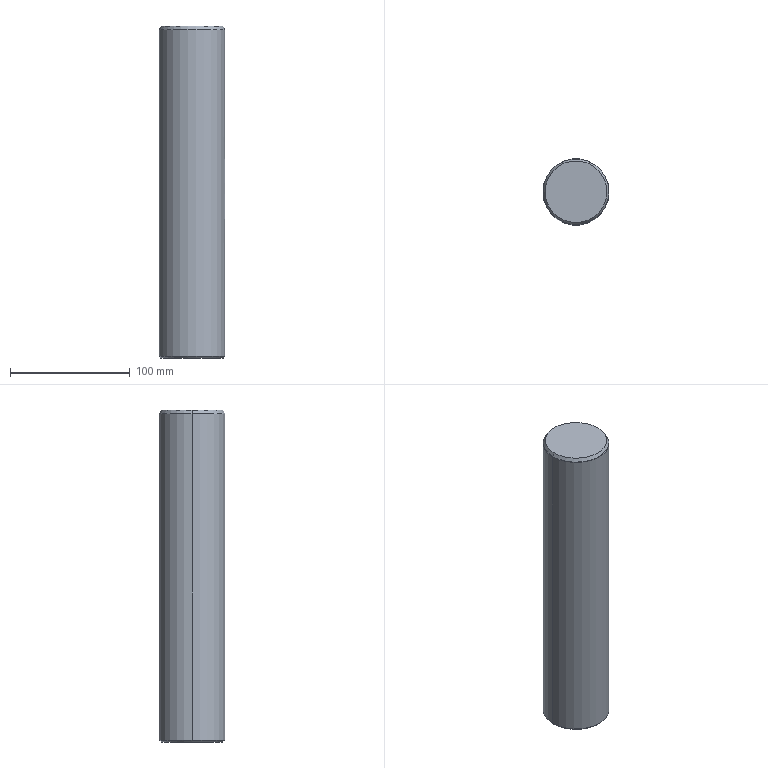Part | SolidWorks | features Chamfer 2, HoleWzd 2, Extrusion 1, Fillet 1 | 1 solid | 22 faces | box 55 x 55 x 277 mm | volume 656436 mm3 | cone 10 | cylinder 8 | torus 2 | plane 2 | commonest cylinder face diameters 6 x4 8 x2 55 x2
STEP:
#1=CARTESIAN_POINT('',(-27.5,0.,273.866));
#2=VERTEX_POINT('',#1);
#3=CARTESIAN_POINT('',(27.5,0.,273.866));
#4=VERTEX_POINT('',#3);
#5=CARTESIAN_POINT('',(0.,0.,273.866));
#6=DIRECTION('',(0.,0.,-1.));
#7=DIRECTION('',(1.,0.,0.));
#8=AXIS2_PLACEMENT_3D('',#5,#6,#7);
#9=CIRCLE('',#8,27.5);
#10=EDGE_CURVE('',#2,#4,#9,.T.);
#11=ORIENTED_EDGE('',*,*,#10,.F.);
#12=CARTESIAN_POINT('',(-27.433,0.,274.116));
#13=VERTEX_POINT('',#12);
#14=CARTESIAN_POINT('',(-27.,0.,273.866));
#15=DIRECTION('',(0.,1.,0.));
#16=DIRECTION('',(-1.,0.,0.));
#17=AXIS2_PLACEMENT_3D('',#14,#15,#16);
#18=CIRCLE('',#17,0.5);
#19=EDGE_CURVE('',#2,#13,#18,.T.);
#20=ORIENTED_EDGE('',*,*,#19,.T.);
#21=CARTESIAN_POINT('',(27.433,0.,274.116));
#22=VERTEX_POINT('',#21);
#23=CARTESIAN_POINT('',(0.,0.,274.116));
#24=DIRECTION('',(0.,0.,1.));
#25=DIRECTION('',(-1.,0.,0.));
#26=AXIS2_PLACEMENT_3D('',#23,#24,#25);
#27=CIRCLE('',#26,27.433);
#28=EDGE_CURVE('',#22,#13,#27,.T.);
#29=ORIENTED_EDGE('',*,*,#28,.F.);
#30=CARTESIAN_POINT('',(27.,0.,273.866));
#31=DIRECTION('',(0.,-1.,0.));
#32=DIRECTION('',(0.,0.,-1.));
#33=AXIS2_PLACEMENT_3D('',#30,#31,#32);
#34=CIRCLE('',#33,0.5);
#35=EDGE_CURVE('',#4,#22,#34,.T.);
#36=ORIENTED_EDGE('',*,*,#35,.F.);
#37=EDGE_LOOP('',(#11,#20,#29,#36));
#38=FACE_OUTER_BOUND('',#37,.T.);
#39=CARTESIAN_POINT('',(0.,0.,273.866));
#40=DIRECTION('',(0.,0.,1.));
#41=DIRECTION('',(1.,0.,0.));
#42=AXIS2_PLACEMENT_3D('',#39,#40,#41);
#43=TOROIDAL_SURFACE('',#42,27.,0.5);
#44=ADVANCED_FACE('',(#38),#43,.T.);
#45=CARTESIAN_POINT('',(25.768,0.,277.));
#46=VERTEX_POINT('',#45);
#47=CARTESIAN_POINT('',(-25.768,0.,277.));
#48=VERTEX_POINT('',#47);
#49=CARTESIAN_POINT('',(0.,0.,277.));
#50=DIRECTION('',(0.,0.,1.));
#51=DIRECTION('',(1.,0.,0.));
#52=AXIS2_PLACEMENT_3D('',#49,#50,#51);
#53=CIRCLE('',#52,25.768);
#54=EDGE_CURVE('',#46,#48,#53,.T.);
#55=ORIENTED_EDGE('',*,*,#54,.F.);
#56=CARTESIAN_POINT('',(25.768,0.,277.));
#57=DIRECTION('',(0.5,0.,-0.866));
#58=VECTOR('',#57,1000.);
#59=LINE('',#56,#58);
#60=EDGE_CURVE('',#46,#22,#59,.T.);
#61=ORIENTED_EDGE('',*,*,#60,.T.);
#62=ORIENTED_EDGE('',*,*,#28,.T.);
#63=CARTESIAN_POINT('',(-25.768,0.,277.));
#64=DIRECTION('',(-0.5,0.,-0.866));
#65=VECTOR('',#64,1000.);
#66=LINE('',#63,#65);
#67=EDGE_CURVE('',#48,#13,#66,.T.);
#68=ORIENTED_EDGE('',*,*,#67,.F.);
#69=EDGE_LOOP('',(#55,#61,#62,#68));
#70=FACE_OUTER_BOUND('',#69,.T.);
#71=CARTESIAN_POINT('',(0.,0.,277.));
#72=DIRECTION('',(0.,0.,-1.));
#73=DIRECTION('',(-1.,0.,0.));
#74=AXIS2_PLACEMENT_3D('',#71,#72,#73);
#75=CONICAL_SURFACE('',#74,25.768,0.5236);
#76=ADVANCED_FACE('',(#70),#75,.T.);
#77=CARTESIAN_POINT('',(-26.,0.,0.));
#78=VERTEX_POINT('',#77);
#79=CARTESIAN_POINT('',(26.,0.,0.));
#80=VERTEX_POINT('',#79);
#81=CARTESIAN_POINT('',(0.,0.,0.));
#82=DIRECTION('',(0.,0.,-1.));
#83=DIRECTION('',(1.,0.,0.));
#84=AXIS2_PLACEMENT_3D('',#81,#82,#83);
#85=CIRCLE('',#84,26.);
#86=EDGE_CURVE('',#78,#80,#85,.T.);
#87=ORIENTED_EDGE('',*,*,#86,.F.);
#88=CARTESIAN_POINT('',(-27.5,0.,1.5));
#89=VERTEX_POINT('',#88);
#90=CARTESIAN_POINT('',(-27.5,0.,1.5));
#91=DIRECTION('',(-0.7071,0.,0.7071));
#92=VECTOR('',#91,1000.);
#93=LINE('',#90,#92);
#94=EDGE_CURVE('',#78,#89,#93,.T.);
#95=ORIENTED_EDGE('',*,*,#94,.T.);
#96=CARTESIAN_POINT('',(27.5,0.,1.5));
#97=VERTEX_POINT('',#96);
#98=CARTESIAN_POINT('',(0.,0.,1.5));
#99=DIRECTION('',(0.,0.,1.));
#100=DIRECTION('',(1.,0.,0.));
#101=AXIS2_PLACEMENT_3D('',#98,#99,#100);
#102=CIRCLE('',#101,27.5);
#103=EDGE_CURVE('',#97,#89,#102,.T.);
#104=ORIENTED_EDGE('',*,*,#103,.F.);
#105=CARTESIAN_POINT('',(27.5,0.,1.5));
#106=DIRECTION('',(0.7071,0.,0.7071));
#107=VECTOR('',#106,1000.);
#108=LINE('',#105,#107);
#109=EDGE_CURVE('',#80,#97,#108,.T.);
#110=ORIENTED_EDGE('',*,*,#109,.F.);
#111=EDGE_LOOP('',(#87,#95,#104,#110));
#112=FACE_OUTER_BOUND('',#111,.T.);
#113=CARTESIAN_POINT('',(0.,0.,1.5));
#114=DIRECTION('',(0.,0.,1.));
#115=DIRECTION('',(1.,0.,0.));
#116=AXIS2_PLACEMENT_3D('',#113,#114,#115);
#117=CONICAL_SURFACE('',#116,27.5,0.7854);
#118=ADVANCED_FACE('',(#112),#117,.T.);
#119=CARTESIAN_POINT('',(17.097,0.,142.));
#120=VERTEX_POINT('',#119);
#121=CARTESIAN_POINT('',(19.5,0.,138.));
#122=VERTEX_POINT('',#121);
#123=CARTESIAN_POINT('',(19.5,0.,138.));
#124=DIRECTION('',(0.515,0.,-0.8572));
#125=VECTOR('',#124,1000.);
#126=LINE('',#123,#125);
#127=EDGE_CURVE('',#120,#122,#126,.T.);
#128=ORIENTED_EDGE('',*,*,#127,.F.);
#129=CARTESIAN_POINT('',(19.5,0.,146.));
#130=VERTEX_POINT('',#129);
#131=CARTESIAN_POINT('',(19.5,0.,146.));
#132=DIRECTION('',(0.515,0.,0.8572));
#133=VECTOR('',#132,1000.);
#134=LINE('',#131,#133);
#135=EDGE_CURVE('',#120,#130,#134,.T.);
#136=ORIENTED_EDGE('',*,*,#135,.T.);
#137=CARTESIAN_POINT('',(19.5,0.,142.));
#138=DIRECTION('',(1.,0.,0.));
#139=DIRECTION('',(0.,0.,-1.));
#140=AXIS2_PLACEMENT_3D('',#137,#138,#139);
#141=CIRCLE('',#140,4.);
#142=EDGE_CURVE('',#130,#122,#141,.T.);
#143=ORIENTED_EDGE('',*,*,#142,.T.);
#144=EDGE_LOOP('',(#128,#136,#143));
#145=FACE_OUTER_BOUND('',#144,.T.);
#146=CARTESIAN_POINT('',(19.5,0.,142.));
#147=DIRECTION('',(1.,0.,0.));
#148=DIRECTION('',(0.,0.,-1.));
#149=AXIS2_PLACEMENT_3D('',#146,#147,#148);
#150=CONICAL_SURFACE('',#149,4.,1.03);
#151=ADVANCED_FACE('',(#145),#150,.F.);
#152=ORIENTED_EDGE('',*,*,#142,.F.);
#153=CARTESIAN_POINT('',(27.5,0.,146.));
#154=VERTEX_POINT('',#153);
#155=CARTESIAN_POINT('',(27.5,0.,146.));
#156=DIRECTION('',(1.,0.,0.));
#157=VECTOR('',#156,1000.);
#158=LINE('',#155,#157);
#159=EDGE_CURVE('',#130,#154,#158,.T.);
#160=ORIENTED_EDGE('',*,*,#159,.T.);
#161=CARTESIAN_POINT('',(27.5,0.,138.));
#162=VERTEX_POINT('',#161);
#163=CARTESIAN_POINT('',(27.5,0.,138.));
#164=CARTESIAN_POINT('',(27.5,-0.2647,138.));
#165=CARTESIAN_POINT('',(27.496,-0.5248,138.026));
#166=CARTESIAN_POINT('',(27.482,-1.037,138.128));
#167=CARTESIAN_POINT('',(27.471,-1.291,138.205));
#168=CARTESIAN_POINT('',(27.444,-1.775,138.406));
#169=CARTESIAN_POINT('',(27.428,-2.005,138.529));
#170=CARTESIAN_POINT('',(27.392,-2.439,138.819));
#171=CARTESIAN_POINT('',(27.373,-2.645,138.988));
#172=CARTESIAN_POINT('',(27.335,-3.013,139.356));
#173=CARTESIAN_POINT('',(27.316,-3.179,139.558));
#174=CARTESIAN_POINT('',(27.28,-3.471,139.995));
#175=CARTESIAN_POINT('',(27.264,-3.595,140.227));
#176=CARTESIAN_POINT('',(27.237,-3.795,140.708));
#177=CARTESIAN_POINT('',(27.226,-3.872,140.961));
#178=CARTESIAN_POINT('',(27.211,-3.974,141.477));
#179=CARTESIAN_POINT('',(27.208,-4.,141.737));
#180=CARTESIAN_POINT('',(27.208,-4.,142.26));
#181=CARTESIAN_POINT('',(27.211,-3.974,142.525));
#182=CARTESIAN_POINT('',(27.226,-3.872,143.039));
#183=CARTESIAN_POINT('',(27.237,-3.796,143.288));
#184=CARTESIAN_POINT('',(27.264,-3.595,143.773));
#185=CARTESIAN_POINT('',(27.281,-3.47,144.006));
#186=CARTESIAN_POINT('',(27.316,-3.181,144.439));
#187=CARTESIAN_POINT('',(27.335,-3.015,144.642));
#188=CARTESIAN_POINT('',(27.373,-2.642,145.015));
#189=CARTESIAN_POINT('',(27.392,-2.44,145.18));
#190=CARTESIAN_POINT('',(27.427,-2.008,145.47));
#191=CARTESIAN_POINT('',(27.444,-1.773,145.595));
#192=CARTESIAN_POINT('',(27.471,-1.289,145.796));
#193=CARTESIAN_POINT('',(27.482,-1.04,145.871));
#194=CARTESIAN_POINT('',(27.496,-0.5266,145.974));
#195=CARTESIAN_POINT('',(27.5,-0.2612,146.));
#196=CARTESIAN_POINT('',(27.5,0.,146.));
#197=B_SPLINE_CURVE_WITH_KNOTS('',3,(#163,#164,#165,#166,#167,#168,#169,#170,#171,#172,#173,#174,#175,#176,#177,#178,#179,#180,#181,#182,#183,#184,#185,#186,#187,#188,#189,#190,#191,#192,#193,#194,#195,#196),.UNSPECIFIED.,.F.,.F.,(4,2,2,2,2,2,2,2,2,2,2,2,2,2,2,2,4),(0.,0.0007827,0.001565,0.002348,0.003131,0.003913,0.004696,0.005479,0.006261,0.007044,0.007827,0.008609,0.009392,0.01017,0.01096,0.01174,0.01252),.UNSPECIFIED.);
#198=EDGE_CURVE('',#162,#154,#197,.T.);
#199=ORIENTED_EDGE('',*,*,#198,.F.);
#200=CARTESIAN_POINT('',(27.5,0.,138.));
#201=DIRECTION('',(1.,0.,0.));
#202=VECTOR('',#201,1000.);
#203=LINE('',#200,#202);
#204=EDGE_CURVE('',#122,#162,#203,.T.);
#205=ORIENTED_EDGE('',*,*,#204,.F.);
#206=EDGE_LOOP('',(#152,#160,#199,#205));
#207=FACE_OUTER_BOUND('',#206,.T.);
#208=CARTESIAN_POINT('',(27.5,0.,142.));
#209=DIRECTION('',(1.,0.,0.));
#210=DIRECTION('',(0.,0.,-1.));
#211=AXIS2_PLACEMENT_3D('',#208,#209,#210);
#212=CYLINDRICAL_SURFACE('',#211,4.);
#213=ADVANCED_FACE('',(#207),#212,.F.);
#214=CARTESIAN_POINT('',(18.,0.,10.));
#215=VERTEX_POINT('',#214);
#216=CARTESIAN_POINT('',(12.,0.,10.));
#217=VERTEX_POINT('',#216);
#218=CARTESIAN_POINT('',(15.,0.,10.));
#219=DIRECTION('',(0.,0.,-1.));
#220=DIRECTION('',(-1.,0.,0.));
#221=AXIS2_PLACEMENT_3D('',#218,#219,#220);
#222=CIRCLE('',#221,3.);
#223=EDGE_CURVE('',#215,#217,#222,.T.);
#224=ORIENTED_EDGE('',*,*,#223,.F.);
#225=CARTESIAN_POINT('',(18.,0.,0.));
#226=VERTEX_POINT('',#225);
#227=CARTESIAN_POINT('',(18.,0.,0.));
#228=DIRECTION('',(0.,0.,-1.));
#229=VECTOR('',#228,1000.);
#230=LINE('',#227,#229);
#231=EDGE_CURVE('',#215,#226,#230,.T.);
#232=ORIENTED_EDGE('',*,*,#231,.T.);
#233=CARTESIAN_POINT('',(12.,0.,0.));
#234=VERTEX_POINT('',#233);
#235=CARTESIAN_POINT('',(15.,0.,0.));
#236=DIRECTION('',(0.,0.,-1.));
#237=DIRECTION('',(-1.,0.,0.));
#238=AXIS2_PLACEMENT_3D('',#235,#236,#237);
#239=CIRCLE('',#238,3.);
#240=EDGE_CURVE('',#226,#234,#239,.T.);
#241=ORIENTED_EDGE('',*,*,#240,.T.);
#242=CARTESIAN_POINT('',(12.,0.,0.));
#243=DIRECTION('',(0.,0.,-1.));
#244=VECTOR('',#243,1000.);
#245=LINE('',#242,#244);
#246=EDGE_CURVE('',#217,#234,#245,.T.);
#247=ORIENTED_EDGE('',*,*,#246,.F.);
#248=EDGE_LOOP('',(#224,#232,#241,#247));
#249=FACE_OUTER_BOUND('',#248,.T.);
#250=CARTESIAN_POINT('',(15.,0.,0.));
#251=DIRECTION('',(0.,0.,-1.));
#252=DIRECTION('',(-1.,0.,0.));
#253=AXIS2_PLACEMENT_3D('',#250,#251,#252);
#254=CYLINDRICAL_SURFACE('',#253,3.);
#255=ADVANCED_FACE('',(#249),#254,.F.);
#256=CARTESIAN_POINT('',(15.,0.,11.803));
#257=VERTEX_POINT('',#256);
#258=CARTESIAN_POINT('',(12.,0.,10.));
#259=DIRECTION('',(-0.8572,0.,-0.515));
#260=VECTOR('',#259,1000.);
#261=LINE('',#258,#260);
#262=EDGE_CURVE('',#257,#217,#261,.T.);
#263=ORIENTED_EDGE('',*,*,#262,.F.);
#264=CARTESIAN_POINT('',(18.,0.,10.));
#265=DIRECTION('',(0.8572,0.,-0.515));
#266=VECTOR('',#265,1000.);
#267=LINE('',#264,#266);
#268=EDGE_CURVE('',#257,#215,#267,.T.);
#269=ORIENTED_EDGE('',*,*,#268,.T.);
#270=ORIENTED_EDGE('',*,*,#223,.T.);
#271=EDGE_LOOP('',(#263,#269,#270));
#272=FACE_OUTER_BOUND('',#271,.T.);
#273=CARTESIAN_POINT('',(15.,0.,10.));
#274=DIRECTION('',(0.,0.,-1.));
#275=DIRECTION('',(-1.,0.,0.));
#276=AXIS2_PLACEMENT_3D('',#273,#274,#275);
#277=CONICAL_SURFACE('',#276,3.,1.03);
#278=ADVANCED_FACE('',(#272),#277,.F.);
#279=CARTESIAN_POINT('',(-12.,0.,10.));
#280=VERTEX_POINT('',#279);
#281=CARTESIAN_POINT('',(-18.,0.,10.));
#282=VERTEX_POINT('',#281);
#283=CARTESIAN_POINT('',(-15.,0.,10.));
#284=DIRECTION('',(0.,0.,-1.));
#285=DIRECTION('',(-1.,0.,0.));
#286=AXIS2_PLACEMENT_3D('',#283,#284,#285);
#287=CIRCLE('',#286,3.);
#288=EDGE_CURVE('',#280,#282,#287,.T.);
#289=ORIENTED_EDGE('',*,*,#288,.F.);
#290=CARTESIAN_POINT('',(-12.,0.,0.));
#291=VERTEX_POINT('',#290);
#292=CARTESIAN_POINT('',(-12.,0.,0.));
#293=DIRECTION('',(0.,0.,-1.));
#294=VECTOR('',#293,1000.);
#295=LINE('',#292,#294);
#296=EDGE_CURVE('',#280,#291,#295,.T.);
#297=ORIENTED_EDGE('',*,*,#296,.T.);
#298=CARTESIAN_POINT('',(-18.,0.,0.));
#299=VERTEX_POINT('',#298);
#300=CARTESIAN_POINT('',(-15.,0.,0.));
#301=DIRECTION('',(0.,0.,-1.));
#302=DIRECTION('',(-1.,0.,0.));
#303=AXIS2_PLACEMENT_3D('',#300,#301,#302);
#304=CIRCLE('',#303,3.);
#305=EDGE_CURVE('',#291,#299,#304,.T.);
#306=ORIENTED_EDGE('',*,*,#305,.T.);
#307=CARTESIAN_POINT('',(-18.,0.,0.));
#308=DIRECTION('',(0.,0.,-1.));
#309=VECTOR('',#308,1000.);
#310=LINE('',#307,#309);
#311=EDGE_CURVE('',#282,#299,#310,.T.);
#312=ORIENTED_EDGE('',*,*,#311,.F.);
#313=EDGE_LOOP('',(#289,#297,#306,#312));
#314=FACE_OUTER_BOUND('',#313,.T.);
#315=CARTESIAN_POINT('',(-15.,0.,0.));
#316=DIRECTION('',(0.,0.,-1.));
#317=DIRECTION('',(-1.,0.,0.));
#318=AXIS2_PLACEMENT_3D('',#315,#316,#317);
#319=CYLINDRICAL_SURFACE('',#318,3.);
#320=ADVANCED_FACE('',(#314),#319,.F.);
#321=CARTESIAN_POINT('',(-15.,0.,11.803));
#322=VERTEX_POINT('',#321);
#323=CARTESIAN_POINT('',(-18.,0.,10.));
#324=DIRECTION('',(-0.8572,0.,-0.515));
#325=VECTOR('',#324,1000.);
#326=LINE('',#323,#325);
#327=EDGE_CURVE('',#322,#282,#326,.T.);
#328=ORIENTED_EDGE('',*,*,#327,.F.);
#329=CARTESIAN_POINT('',(-12.,0.,10.));
#330=DIRECTION('',(0.8572,0.,-0.515));
#331=VECTOR('',#330,1000.);
#332=LINE('',#329,#331);
#333=EDGE_CURVE('',#322,#280,#332,.T.);
#334=ORIENTED_EDGE('',*,*,#333,.T.);
#335=ORIENTED_EDGE('',*,*,#288,.T.);
#336=EDGE_LOOP('',(#328,#334,#335));
#337=FACE_OUTER_BOUND('',#336,.T.);
#338=CARTESIAN_POINT('',(-15.,0.,10.));
#339=DIRECTION('',(0.,0.,-1.));
#340=DIRECTION('',(-1.,0.,0.));
#341=AXIS2_PLACEMENT_3D('',#338,#339,#340);
#342=CONICAL_SURFACE('',#341,3.,1.03);
#343=ADVANCED_FACE('',(#337),#342,.F.);
#344=ORIENTED_EDGE('',*,*,#10,.T.);
#345=CARTESIAN_POINT('',(27.5,0.,277.));
#346=DIRECTION('',(0.,0.,-1.));
#347=VECTOR('',#346,1000.);
#348=LINE('',#345,#347);
#349=EDGE_CURVE('',#4,#154,#348,.T.);
#350=ORIENTED_EDGE('',*,*,#349,.T.);
#351=CARTESIAN_POINT('',(27.5,0.,146.));
#352=CARTESIAN_POINT('',(27.5,0.2612,146.));
#353=CARTESIAN_POINT('',(27.496,0.521,145.975));
#354=CARTESIAN_POINT('',(27.482,1.038,145.872));
#355=CARTESIAN_POINT('',(27.471,1.29,145.795));
#356=CARTESIAN_POINT('',(27.444,1.771,145.596));
#357=CARTESIAN_POINT('',(27.428,2.004,145.472));
#358=CARTESIAN_POINT('',(27.392,2.441,145.18));
#359=CARTESIAN_POINT('',(27.373,2.642,145.014));
#360=CARTESIAN_POINT('',(27.335,3.011,144.646));
#361=CARTESIAN_POINT('',(27.316,3.18,144.441));
#362=CARTESIAN_POINT('',(27.281,3.47,144.007));
#363=CARTESIAN_POINT('',(27.264,3.593,143.777));
#364=CARTESIAN_POINT('',(27.237,3.794,143.293));
#365=CARTESIAN_POINT('',(27.226,3.871,143.039));
#366=CARTESIAN_POINT('',(27.211,3.974,142.528));
#367=CARTESIAN_POINT('',(27.208,4.,142.267));
#368=CARTESIAN_POINT('',(27.208,4.,141.738));
#369=CARTESIAN_POINT('',(27.211,3.974,141.478));
#370=CARTESIAN_POINT('',(27.226,3.873,140.966));
#371=CARTESIAN_POINT('',(27.237,3.796,140.712));
#372=CARTESIAN_POINT('',(27.264,3.596,140.228));
#373=CARTESIAN_POINT('',(27.28,3.473,139.998));
#374=CARTESIAN_POINT('',(27.316,3.183,139.563));
#375=CARTESIAN_POINT('',(27.335,3.014,139.358));
#376=CARTESIAN_POINT('',(27.373,2.646,138.989));
#377=CARTESIAN_POINT('',(27.392,2.445,138.824));
#378=CARTESIAN_POINT('',(27.427,2.008,138.531));
#379=CARTESIAN_POINT('',(27.444,1.776,138.407));
#380=CARTESIAN_POINT('',(27.471,1.295,138.207));
#381=CARTESIAN_POINT('',(27.481,1.043,138.129));
#382=CARTESIAN_POINT('',(27.496,0.5261,138.026));
#383=CARTESIAN_POINT('',(27.5,0.2646,138.));
#384=CARTESIAN_POINT('',(27.5,0.,138.));
#385=B_SPLINE_CURVE_WITH_KNOTS('',3,(#351,#352,#353,#354,#355,#356,#357,#358,#359,#360,#361,#362,#363,#364,#365,#366,#367,#368,#369,#370,#371,#372,#373,#374,#375,#376,#377,#378,#379,#380,#381,#382,#383,#384),.UNSPECIFIED.,.F.,.F.,(4,2,2,2,2,2,2,2,2,2,2,2,2,2,2,2,4),(0.01252,0.0133,0.01409,0.01487,0.01565,0.01643,0.01722,0.018,0.01878,0.01956,0.02035,0.02113,0.02191,0.02269,0.02348,0.02426,0.02504),.UNSPECIFIED.);
#386=EDGE_CURVE('',#154,#162,#385,.T.);
#387=ORIENTED_EDGE('',*,*,#386,.T.);
#388=CARTESIAN_POINT('',(27.5,0.,277.));
#389=DIRECTION('',(0.,0.,-1.));
#390=VECTOR('',#389,1000.);
#391=LINE('',#388,#390);
#392=EDGE_CURVE('',#162,#97,#391,.T.);
#393=ORIENTED_EDGE('',*,*,#392,.T.);
#394=ORIENTED_EDGE('',*,*,#103,.T.);
#395=CARTESIAN_POINT('',(-27.5,0.,277.));
#396=DIRECTION('',(0.,0.,-1.));
#397=VECTOR('',#396,1000.);
#398=LINE('',#395,#397);
#399=EDGE_CURVE('',#2,#89,#398,.T.);
#400=ORIENTED_EDGE('',*,*,#399,.F.);
#401=EDGE_LOOP('',(#344,#350,#387,#393,#394,#400));
#402=FACE_OUTER_BOUND('',#401,.T.);
#403=CARTESIAN_POINT('',(0.,0.,277.));
#404=DIRECTION('',(0.,0.,-1.));
#405=DIRECTION('',(-1.,0.,0.));
#406=AXIS2_PLACEMENT_3D('',#403,#404,#405);
#407=CYLINDRICAL_SURFACE('',#406,27.5);
#408=ADVANCED_FACE('',(#402),#407,.T.);
#409=ORIENTED_EDGE('',*,*,#349,.F.);
#410=CARTESIAN_POINT('',(0.,0.,273.866));
#411=DIRECTION('',(0.,0.,-1.));
#412=DIRECTION('',(1.,0.,0.));
#413=AXIS2_PLACEMENT_3D('',#410,#411,#412);
#414=CIRCLE('',#413,27.5);
#415=EDGE_CURVE('',#4,#2,#414,.T.);
#416=ORIENTED_EDGE('',*,*,#415,.T.);
#417=ORIENTED_EDGE('',*,*,#399,.T.);
#418=CARTESIAN_POINT('',(0.,0.,1.5));
#419=DIRECTION('',(0.,0.,1.));
#420=DIRECTION('',(1.,0.,0.));
#421=AXIS2_PLACEMENT_3D('',#418,#419,#420);
#422=CIRCLE('',#421,27.5);
#423=EDGE_CURVE('',#89,#97,#422,.T.);
#424=ORIENTED_EDGE('',*,*,#423,.T.);
#425=ORIENTED_EDGE('',*,*,#392,.F.);
#426=ORIENTED_EDGE('',*,*,#198,.T.);
#427=EDGE_LOOP('',(#409,#416,#417,#424,#425,#426));
#428=FACE_OUTER_BOUND('',#427,.T.);
#429=CARTESIAN_POINT('',(0.,0.,277.));
#430=DIRECTION('',(0.,0.,-1.));
#431=DIRECTION('',(-1.,0.,0.));
#432=AXIS2_PLACEMENT_3D('',#429,#430,#431);
#433=CYLINDRICAL_SURFACE('',#432,27.5);
#434=ADVANCED_FACE('',(#428),#433,.T.);
#435=CARTESIAN_POINT('',(0.,0.,277.));
#436=DIRECTION('',(0.,0.,1.));
#437=DIRECTION('',(1.,0.,0.));
#438=AXIS2_PLACEMENT_3D('',#435,#436,#437);
#439=CIRCLE('',#438,25.768);
#440=EDGE_CURVE('',#48,#46,#439,.T.);
#441=ORIENTED_EDGE('',*,*,#440,.T.);
#442=ORIENTED_EDGE('',*,*,#54,.T.);
#443=EDGE_LOOP('',(#441,#442));
#444=FACE_OUTER_BOUND('',#443,.T.);
#445=CARTESIAN_POINT('',(0.,0.,277.));
#446=DIRECTION('',(0.,0.,1.));
#447=DIRECTION('',(1.,0.,0.));
#448=AXIS2_PLACEMENT_3D('',#445,#446,#447);
#449=PLANE('',#448);
#450=ADVANCED_FACE('',(#444),#449,.T.);
#451=CARTESIAN_POINT('',(0.,0.,0.));
#452=DIRECTION('',(0.,0.,-1.));
#453=DIRECTION('',(1.,0.,0.));
#454=AXIS2_PLACEMENT_3D('',#451,#452,#453);
#455=CIRCLE('',#454,26.);
#456=EDGE_CURVE('',#80,#78,#455,.T.);
#457=ORIENTED_EDGE('',*,*,#456,.T.);
#458=ORIENTED_EDGE('',*,*,#86,.T.);
#459=EDGE_LOOP('',(#457,#458));
#460=FACE_OUTER_BOUND('',#459,.T.);
#461=CARTESIAN_POINT('',(15.,0.,0.));
#462=DIRECTION('',(0.,0.,-1.));
#463=DIRECTION('',(-1.,0.,0.));
#464=AXIS2_PLACEMENT_3D('',#461,#462,#463);
#465=CIRCLE('',#464,3.);
#466=EDGE_CURVE('',#234,#226,#465,.T.);
#467=ORIENTED_EDGE('',*,*,#466,.F.);
#468=ORIENTED_EDGE('',*,*,#240,.F.);
#469=EDGE_LOOP('',(#467,#468));
#470=FACE_BOUND('',#469,.T.);
#471=CARTESIAN_POINT('',(-15.,0.,0.));
#472=DIRECTION('',(0.,0.,-1.));
#473=DIRECTION('',(-1.,0.,0.));
#474=AXIS2_PLACEMENT_3D('',#471,#472,#473);
#475=CIRCLE('',#474,3.);
#476=EDGE_CURVE('',#299,#291,#475,.T.);
#477=ORIENTED_EDGE('',*,*,#476,.F.);
#478=ORIENTED_EDGE('',*,*,#305,.F.);
#479=EDGE_LOOP('',(#477,#478));
#480=FACE_BOUND('',#479,.T.);
#481=CARTESIAN_POINT('',(0.,0.,0.));
#482=DIRECTION('',(0.,0.,1.));
#483=DIRECTION('',(1.,0.,0.));
#484=AXIS2_PLACEMENT_3D('',#481,#482,#483);
#485=PLANE('',#484);
#486=ADVANCED_FACE('',(#460,#470,#480),#485,.F.);
#487=ORIENTED_EDGE('',*,*,#333,.F.);
#488=ORIENTED_EDGE('',*,*,#327,.T.);
#489=CARTESIAN_POINT('',(-15.,0.,10.));
#490=DIRECTION('',(0.,0.,-1.));
#491=DIRECTION('',(-1.,0.,0.));
#492=AXIS2_PLACEMENT_3D('',#489,#490,#491);
#493=CIRCLE('',#492,3.);
#494=EDGE_CURVE('',#282,#280,#493,.T.);
#495=ORIENTED_EDGE('',*,*,#494,.T.);
#496=EDGE_LOOP('',(#487,#488,#495));
#497=FACE_OUTER_BOUND('',#496,.T.);
#498=CARTESIAN_POINT('',(-15.,0.,10.));
#499=DIRECTION('',(0.,0.,-1.));
#500=DIRECTION('',(-1.,0.,0.));
#501=AXIS2_PLACEMENT_3D('',#498,#499,#500);
#502=CONICAL_SURFACE('',#501,3.,1.03);
#503=ADVANCED_FACE('',(#497),#502,.F.);
#504=ORIENTED_EDGE('',*,*,#296,.F.);
#505=ORIENTED_EDGE('',*,*,#494,.F.);
#506=ORIENTED_EDGE('',*,*,#311,.T.);
#507=ORIENTED_EDGE('',*,*,#476,.T.);
#508=EDGE_LOOP('',(#504,#505,#506,#507));
#509=FACE_OUTER_BOUND('',#508,.T.);
#510=CARTESIAN_POINT('',(-15.,0.,0.));
#511=DIRECTION('',(0.,0.,-1.));
#512=DIRECTION('',(-1.,0.,0.));
#513=AXIS2_PLACEMENT_3D('',#510,#511,#512);
#514=CYLINDRICAL_SURFACE('',#513,3.);
#515=ADVANCED_FACE('',(#509),#514,.F.);
#516=ORIENTED_EDGE('',*,*,#268,.F.);
#517=ORIENTED_EDGE('',*,*,#262,.T.);
#518=CARTESIAN_POINT('',(15.,0.,10.));
#519=DIRECTION('',(0.,0.,-1.));
#520=DIRECTION('',(-1.,0.,0.));
#521=AXIS2_PLACEMENT_3D('',#518,#519,#520);
#522=CIRCLE('',#521,3.);
#523=EDGE_CURVE('',#217,#215,#522,.T.);
#524=ORIENTED_EDGE('',*,*,#523,.T.);
#525=EDGE_LOOP('',(#516,#517,#524));
#526=FACE_OUTER_BOUND('',#525,.T.);
#527=CARTESIAN_POINT('',(15.,0.,10.));
#528=DIRECTION('',(0.,0.,-1.));
#529=DIRECTION('',(-1.,0.,0.));
#530=AXIS2_PLACEMENT_3D('',#527,#528,#529);
#531=CONICAL_SURFACE('',#530,3.,1.03);
#532=ADVANCED_FACE('',(#526),#531,.F.);
#533=ORIENTED_EDGE('',*,*,#231,.F.);
#534=ORIENTED_EDGE('',*,*,#523,.F.);
#535=ORIENTED_EDGE('',*,*,#246,.T.);
#536=ORIENTED_EDGE('',*,*,#466,.T.);
#537=EDGE_LOOP('',(#533,#534,#535,#536));
#538=FACE_OUTER_BOUND('',#537,.T.);
#539=CARTESIAN_POINT('',(15.,0.,0.));
#540=DIRECTION('',(0.,0.,-1.));
#541=DIRECTION('',(-1.,0.,0.));
#542=AXIS2_PLACEMENT_3D('',#539,#540,#541);
#543=CYLINDRICAL_SURFACE('',#542,3.);
#544=ADVANCED_FACE('',(#538),#543,.F.);
#545=ORIENTED_EDGE('',*,*,#159,.F.);
#546=CARTESIAN_POINT('',(19.5,0.,142.));
#547=DIRECTION('',(1.,0.,0.));
#548=DIRECTION('',(0.,0.,-1.));
#549=AXIS2_PLACEMENT_3D('',#546,#547,#548);
#550=CIRCLE('',#549,4.);
#551=EDGE_CURVE('',#122,#130,#550,.T.);
#552=ORIENTED_EDGE('',*,*,#551,.F.);
#553=ORIENTED_EDGE('',*,*,#204,.T.);
#554=ORIENTED_EDGE('',*,*,#386,.F.);
#555=EDGE_LOOP('',(#545,#552,#553,#554));
#556=FACE_OUTER_BOUND('',#555,.T.);
#557=CARTESIAN_POINT('',(27.5,0.,142.));
#558=DIRECTION('',(1.,0.,0.));
#559=DIRECTION('',(0.,0.,-1.));
#560=AXIS2_PLACEMENT_3D('',#557,#558,#559);
#561=CYLINDRICAL_SURFACE('',#560,4.);
#562=ADVANCED_FACE('',(#556),#561,.F.);
#563=ORIENTED_EDGE('',*,*,#135,.F.);
#564=ORIENTED_EDGE('',*,*,#127,.T.);
#565=ORIENTED_EDGE('',*,*,#551,.T.);
#566=EDGE_LOOP('',(#563,#564,#565));
#567=FACE_OUTER_BOUND('',#566,.T.);
#568=CARTESIAN_POINT('',(19.5,0.,142.));
#569=DIRECTION('',(1.,0.,0.));
#570=DIRECTION('',(0.,0.,-1.));
#571=AXIS2_PLACEMENT_3D('',#568,#569,#570);
#572=CONICAL_SURFACE('',#571,4.,1.03);
#573=ADVANCED_FACE('',(#567),#572,.F.);
#574=ORIENTED_EDGE('',*,*,#94,.F.);
#575=ORIENTED_EDGE('',*,*,#456,.F.);
#576=ORIENTED_EDGE('',*,*,#109,.T.);
#577=ORIENTED_EDGE('',*,*,#423,.F.);
#578=EDGE_LOOP('',(#574,#575,#576,#577));
#579=FACE_OUTER_BOUND('',#578,.T.);
#580=CARTESIAN_POINT('',(0.,0.,1.5));
#581=DIRECTION('',(0.,0.,1.));
#582=DIRECTION('',(1.,0.,0.));
#583=AXIS2_PLACEMENT_3D('',#580,#581,#582);
#584=CONICAL_SURFACE('',#583,27.5,0.7854);
#585=ADVANCED_FACE('',(#579),#584,.T.);
#586=ORIENTED_EDGE('',*,*,#60,.F.);
#587=ORIENTED_EDGE('',*,*,#440,.F.);
#588=ORIENTED_EDGE('',*,*,#67,.T.);
#589=CARTESIAN_POINT('',(0.,0.,274.116));
#590=DIRECTION('',(0.,0.,1.));
#591=DIRECTION('',(-1.,0.,0.));
#592=AXIS2_PLACEMENT_3D('',#589,#590,#591);
#593=CIRCLE('',#592,27.433);
#594=EDGE_CURVE('',#13,#22,#593,.T.);
#595=ORIENTED_EDGE('',*,*,#594,.T.);
#596=EDGE_LOOP('',(#586,#587,#588,#595));
#597=FACE_OUTER_BOUND('',#596,.T.);
#598=CARTESIAN_POINT('',(0.,0.,277.));
#599=DIRECTION('',(0.,0.,-1.));
#600=DIRECTION('',(-1.,0.,0.));
#601=AXIS2_PLACEMENT_3D('',#598,#599,#600);
#602=CONICAL_SURFACE('',#601,25.768,0.5236);
#603=ADVANCED_FACE('',(#597),#602,.T.);
#604=ORIENTED_EDGE('',*,*,#19,.F.);
#605=ORIENTED_EDGE('',*,*,#415,.F.);
#606=ORIENTED_EDGE('',*,*,#35,.T.);
#607=ORIENTED_EDGE('',*,*,#594,.F.);
#608=EDGE_LOOP('',(#604,#605,#606,#607));
#609=FACE_OUTER_BOUND('',#608,.T.);
#610=CARTESIAN_POINT('',(0.,0.,273.866));
#611=DIRECTION('',(0.,0.,1.));
#612=DIRECTION('',(1.,0.,0.));
#613=AXIS2_PLACEMENT_3D('',#610,#611,#612);
#614=TOROIDAL_SURFACE('',#613,27.,0.5);
#615=ADVANCED_FACE('',(#609),#614,.T.);
#616=CLOSED_SHELL('',(#44,#76,#118,#151,#213,#255,#278,#320,#343,#408,#434,#450,#486,#503,#515,#532,#544,#562,#573,#585,#603,#615));
#617=MANIFOLD_SOLID_BREP('',#616);
#618=CARTESIAN_POINT('',(0.,0.,0.));
#619=DIRECTION('',(0.,0.,1.));
#620=DIRECTION('',(1.,0.,0.));
#621=AXIS2_PLACEMENT_3D('',#618,#619,#620);
#622=(LENGTH_UNIT()NAMED_UNIT(*)SI_UNIT(.MILLI.,.METRE.));
#623=UNCERTAINTY_MEASURE_WITH_UNIT(LENGTH_MEASURE(0.00001),#622,'','');
#624=(NAMED_UNIT(*)PLANE_ANGLE_UNIT()SI_UNIT($,.RADIAN.));
#625=(NAMED_UNIT(*)SI_UNIT($,.STERADIAN.)SOLID_ANGLE_UNIT());
#626=(GEOMETRIC_REPRESENTATION_CONTEXT(3)GLOBAL_UNCERTAINTY_ASSIGNED_CONTEXT((#623))GLOBAL_UNIT_ASSIGNED_CONTEXT((#622,#624,#625))REPRESENTATION_CONTEXT('',''));
#627=ADVANCED_BREP_SHAPE_REPRESENTATION('',(#617,#621),#626);